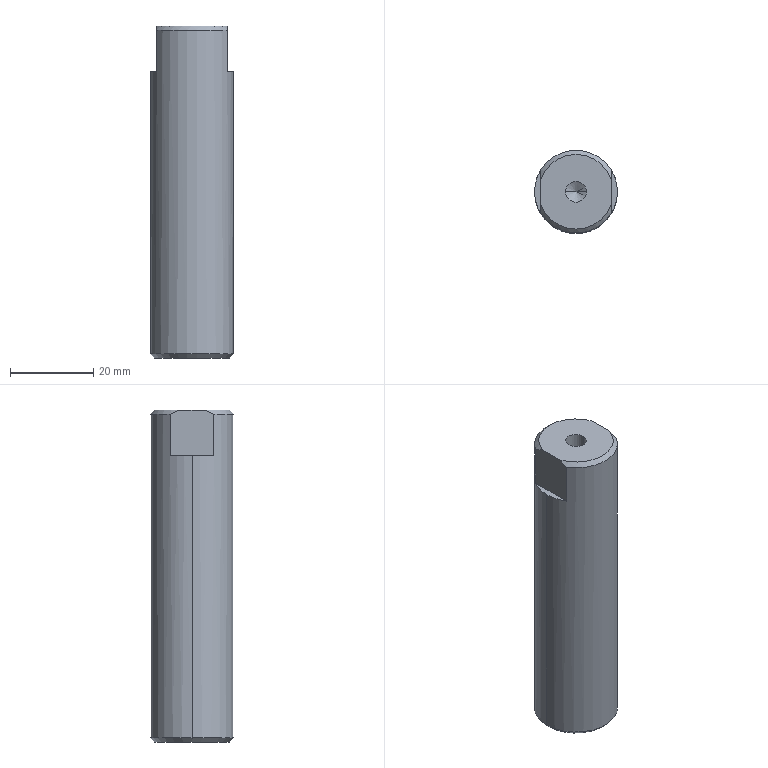Part | STEP file | MT-COMBO-119-S009 | 1 solid | 20 faces | box 20 x 20 x 80 mm | volume 24237 mm3 | cone 8 | cylinder 6 | plane 6 | commonest cylinder face diameters 5 x4 20 x2
STEP:
#1=CARTESIAN_POINT('',(2.5,0.,-65.));
#2=VERTEX_POINT('',#1);
#3=CARTESIAN_POINT('',(-2.5,0.,-65.));
#4=VERTEX_POINT('',#3);
#5=CARTESIAN_POINT('',(0.,0.,-65.));
#6=DIRECTION('',(0.,0.,-1.));
#7=DIRECTION('',(-1.,0.,0.));
#8=AXIS2_PLACEMENT_3D('',#5,#6,#7);
#9=CIRCLE('',#8,2.5);
#10=EDGE_CURVE('',#2,#4,#9,.T.);
#11=ORIENTED_EDGE('',*,*,#10,.F.);
#12=CARTESIAN_POINT('',(2.5,0.,-80.));
#13=VERTEX_POINT('',#12);
#14=CARTESIAN_POINT('',(2.5,0.,-80.));
#15=DIRECTION('',(0.,0.,-1.));
#16=VECTOR('',#15,1000.);
#17=LINE('',#14,#16);
#18=EDGE_CURVE('',#2,#13,#17,.T.);
#19=ORIENTED_EDGE('',*,*,#18,.T.);
#20=CARTESIAN_POINT('',(-2.5,0.,-80.));
#21=VERTEX_POINT('',#20);
#22=CARTESIAN_POINT('',(0.,0.,-80.));
#23=DIRECTION('',(0.,0.,-1.));
#24=DIRECTION('',(-1.,0.,0.));
#25=AXIS2_PLACEMENT_3D('',#22,#23,#24);
#26=CIRCLE('',#25,2.5);
#27=EDGE_CURVE('',#13,#21,#26,.T.);
#28=ORIENTED_EDGE('',*,*,#27,.T.);
#29=CARTESIAN_POINT('',(-2.5,0.,-80.));
#30=DIRECTION('',(0.,0.,-1.));
#31=VECTOR('',#30,1000.);
#32=LINE('',#29,#31);
#33=EDGE_CURVE('',#4,#21,#32,.T.);
#34=ORIENTED_EDGE('',*,*,#33,.F.);
#35=EDGE_LOOP('',(#11,#19,#28,#34));
#36=FACE_OUTER_BOUND('',#35,.T.);
#37=CARTESIAN_POINT('',(0.,0.,-80.));
#38=DIRECTION('',(0.,0.,-1.));
#39=DIRECTION('',(-1.,0.,0.));
#40=AXIS2_PLACEMENT_3D('',#37,#38,#39);
#41=CYLINDRICAL_SURFACE('',#40,2.5);
#42=ADVANCED_FACE('',(#36),#41,.F.);
#43=CARTESIAN_POINT('',(0.,0.,-63.498));
#44=VERTEX_POINT('',#43);
#45=CARTESIAN_POINT('',(-2.5,0.,-65.));
#46=DIRECTION('',(-0.8572,0.,-0.515));
#47=VECTOR('',#46,1000.);
#48=LINE('',#45,#47);
#49=EDGE_CURVE('',#44,#4,#48,.T.);
#50=ORIENTED_EDGE('',*,*,#49,.F.);
#51=CARTESIAN_POINT('',(2.5,0.,-65.));
#52=DIRECTION('',(0.8572,0.,-0.515));
#53=VECTOR('',#52,1000.);
#54=LINE('',#51,#53);
#55=EDGE_CURVE('',#44,#2,#54,.T.);
#56=ORIENTED_EDGE('',*,*,#55,.T.);
#57=ORIENTED_EDGE('',*,*,#10,.T.);
#58=EDGE_LOOP('',(#50,#56,#57));
#59=FACE_OUTER_BOUND('',#58,.T.);
#60=CARTESIAN_POINT('',(0.,0.,-65.));
#61=DIRECTION('',(0.,0.,-1.));
#62=DIRECTION('',(-1.,0.,0.));
#63=AXIS2_PLACEMENT_3D('',#60,#61,#62);
#64=CONICAL_SURFACE('',#63,2.5,1.03);
#65=ADVANCED_FACE('',(#59),#64,.F.);
#66=CARTESIAN_POINT('',(-2.5,0.,-15.));
#67=VERTEX_POINT('',#66);
#68=CARTESIAN_POINT('',(2.5,0.,-15.));
#69=VERTEX_POINT('',#68);
#70=CARTESIAN_POINT('',(0.,0.,-15.));
#71=DIRECTION('',(0.,0.,1.));
#72=DIRECTION('',(1.,0.,0.));
#73=AXIS2_PLACEMENT_3D('',#70,#71,#72);
#74=CIRCLE('',#73,2.5);
#75=EDGE_CURVE('',#67,#69,#74,.T.);
#76=ORIENTED_EDGE('',*,*,#75,.F.);
#77=CARTESIAN_POINT('',(-2.5,0.,0.));
#78=VERTEX_POINT('',#77);
#79=CARTESIAN_POINT('',(-2.5,0.,0.));
#80=DIRECTION('',(0.,0.,1.));
#81=VECTOR('',#80,1000.);
#82=LINE('',#79,#81);
#83=EDGE_CURVE('',#67,#78,#82,.T.);
#84=ORIENTED_EDGE('',*,*,#83,.T.);
#85=CARTESIAN_POINT('',(2.5,0.,0.));
#86=VERTEX_POINT('',#85);
#87=CARTESIAN_POINT('',(0.,0.,0.));
#88=DIRECTION('',(0.,0.,1.));
#89=DIRECTION('',(1.,0.,0.));
#90=AXIS2_PLACEMENT_3D('',#87,#88,#89);
#91=CIRCLE('',#90,2.5);
#92=EDGE_CURVE('',#78,#86,#91,.T.);
#93=ORIENTED_EDGE('',*,*,#92,.T.);
#94=CARTESIAN_POINT('',(2.5,0.,0.));
#95=DIRECTION('',(0.,0.,1.));
#96=VECTOR('',#95,1000.);
#97=LINE('',#94,#96);
#98=EDGE_CURVE('',#69,#86,#97,.T.);
#99=ORIENTED_EDGE('',*,*,#98,.F.);
#100=EDGE_LOOP('',(#76,#84,#93,#99));
#101=FACE_OUTER_BOUND('',#100,.T.);
#102=CARTESIAN_POINT('',(0.,0.,0.));
#103=DIRECTION('',(0.,0.,1.));
#104=DIRECTION('',(1.,0.,0.));
#105=AXIS2_PLACEMENT_3D('',#102,#103,#104);
#106=CYLINDRICAL_SURFACE('',#105,2.5);
#107=ADVANCED_FACE('',(#101),#106,.F.);
#108=CARTESIAN_POINT('',(0.,0.,-16.502));
#109=VERTEX_POINT('',#108);
#110=CARTESIAN_POINT('',(2.5,0.,-15.));
#111=DIRECTION('',(0.8572,0.,0.515));
#112=VECTOR('',#111,1000.);
#113=LINE('',#110,#112);
#114=EDGE_CURVE('',#109,#69,#113,.T.);
#115=ORIENTED_EDGE('',*,*,#114,.F.);
#116=CARTESIAN_POINT('',(-2.5,0.,-15.));
#117=DIRECTION('',(-0.8572,0.,0.515));
#118=VECTOR('',#117,1000.);
#119=LINE('',#116,#118);
#120=EDGE_CURVE('',#109,#67,#119,.T.);
#121=ORIENTED_EDGE('',*,*,#120,.T.);
#122=ORIENTED_EDGE('',*,*,#75,.T.);
#123=EDGE_LOOP('',(#115,#121,#122));
#124=FACE_OUTER_BOUND('',#123,.T.);
#125=CARTESIAN_POINT('',(0.,0.,-15.));
#126=DIRECTION('',(0.,0.,1.));
#127=DIRECTION('',(1.,0.,0.));
#128=AXIS2_PLACEMENT_3D('',#125,#126,#127);
#129=CONICAL_SURFACE('',#128,2.5,1.03);
#130=ADVANCED_FACE('',(#124),#129,.F.);
#131=CARTESIAN_POINT('',(10.,0.,-79.));
#132=VERTEX_POINT('',#131);
#133=CARTESIAN_POINT('',(-10.,0.,-79.));
#134=VERTEX_POINT('',#133);
#135=CARTESIAN_POINT('',(0.,0.,-79.));
#136=DIRECTION('',(0.,0.,-1.));
#137=DIRECTION('',(-1.,0.,0.));
#138=AXIS2_PLACEMENT_3D('',#135,#136,#137);
#139=CIRCLE('',#138,10.);
#140=EDGE_CURVE('',#132,#134,#139,.T.);
#141=ORIENTED_EDGE('',*,*,#140,.F.);
#142=CARTESIAN_POINT('',(10.,0.,-11.));
#143=VERTEX_POINT('',#142);
#144=CARTESIAN_POINT('',(10.,0.,-80.));
#145=DIRECTION('',(0.,0.,1.));
#146=VECTOR('',#145,1000.);
#147=LINE('',#144,#146);
#148=EDGE_CURVE('',#132,#143,#147,.T.);
#149=ORIENTED_EDGE('',*,*,#148,.T.);
#150=CARTESIAN_POINT('',(8.5,-5.268,-11.));
#151=VERTEX_POINT('',#150);
#152=CARTESIAN_POINT('',(0.,0.,-11.));
#153=DIRECTION('',(0.,0.,1.));
#154=DIRECTION('',(1.,0.,0.));
#155=AXIS2_PLACEMENT_3D('',#152,#153,#154);
#156=CIRCLE('',#155,10.);
#157=EDGE_CURVE('',#151,#143,#156,.T.);
#158=ORIENTED_EDGE('',*,*,#157,.F.);
#159=CARTESIAN_POINT('',(8.5,-5.268,-1.));
#160=VERTEX_POINT('',#159);
#161=CARTESIAN_POINT('',(8.5,-5.268,-11.));
#162=DIRECTION('',(0.,0.,1.));
#163=VECTOR('',#162,1000.);
#164=LINE('',#161,#163);
#165=EDGE_CURVE('',#151,#160,#164,.T.);
#166=ORIENTED_EDGE('',*,*,#165,.T.);
#167=CARTESIAN_POINT('',(-8.5,-5.268,-1.));
#168=VERTEX_POINT('',#167);
#169=CARTESIAN_POINT('',(0.,0.,-1.));
#170=DIRECTION('',(0.,0.,-1.));
#171=DIRECTION('',(-1.,0.,0.));
#172=AXIS2_PLACEMENT_3D('',#169,#170,#171);
#173=CIRCLE('',#172,10.);
#174=EDGE_CURVE('',#160,#168,#173,.T.);
#175=ORIENTED_EDGE('',*,*,#174,.T.);
#176=CARTESIAN_POINT('',(-8.5,-5.268,-11.));
#177=VERTEX_POINT('',#176);
#178=CARTESIAN_POINT('',(-8.5,-5.268,-11.));
#179=DIRECTION('',(0.,0.,1.));
#180=VECTOR('',#179,1000.);
#181=LINE('',#178,#180);
#182=EDGE_CURVE('',#177,#168,#181,.T.);
#183=ORIENTED_EDGE('',*,*,#182,.F.);
#184=CARTESIAN_POINT('',(-10.,0.,-11.));
#185=VERTEX_POINT('',#184);
#186=CARTESIAN_POINT('',(0.,0.,-11.));
#187=DIRECTION('',(0.,0.,1.));
#188=DIRECTION('',(1.,0.,0.));
#189=AXIS2_PLACEMENT_3D('',#186,#187,#188);
#190=CIRCLE('',#189,10.);
#191=EDGE_CURVE('',#185,#177,#190,.T.);
#192=ORIENTED_EDGE('',*,*,#191,.F.);
#193=CARTESIAN_POINT('',(-10.,0.,-80.));
#194=DIRECTION('',(0.,0.,1.));
#195=VECTOR('',#194,1000.);
#196=LINE('',#193,#195);
#197=EDGE_CURVE('',#134,#185,#196,.T.);
#198=ORIENTED_EDGE('',*,*,#197,.F.);
#199=EDGE_LOOP('',(#141,#149,#158,#166,#175,#183,#192,#198));
#200=FACE_OUTER_BOUND('',#199,.T.);
#201=CARTESIAN_POINT('',(0.,0.,-80.));
#202=DIRECTION('',(0.,0.,1.));
#203=DIRECTION('',(-1.,0.,0.));
#204=AXIS2_PLACEMENT_3D('',#201,#202,#203);
#205=CYLINDRICAL_SURFACE('',#204,10.);
#206=ADVANCED_FACE('',(#200),#205,.T.);
#207=CARTESIAN_POINT('',(-9.,0.,-80.));
#208=VERTEX_POINT('',#207);
#209=CARTESIAN_POINT('',(9.,0.,-80.));
#210=VERTEX_POINT('',#209);
#211=CARTESIAN_POINT('',(0.,0.,-80.));
#212=DIRECTION('',(0.,0.,-1.));
#213=DIRECTION('',(-1.,0.,0.));
#214=AXIS2_PLACEMENT_3D('',#211,#212,#213);
#215=CIRCLE('',#214,9.);
#216=EDGE_CURVE('',#208,#210,#215,.T.);
#217=ORIENTED_EDGE('',*,*,#216,.F.);
#218=CARTESIAN_POINT('',(-10.,0.,-79.));
#219=DIRECTION('',(-0.7071,0.,0.7071));
#220=VECTOR('',#219,1000.);
#221=LINE('',#218,#220);
#222=EDGE_CURVE('',#208,#134,#221,.T.);
#223=ORIENTED_EDGE('',*,*,#222,.T.);
#224=CARTESIAN_POINT('',(0.,0.,-79.));
#225=DIRECTION('',(0.,0.,-1.));
#226=DIRECTION('',(-1.,0.,0.));
#227=AXIS2_PLACEMENT_3D('',#224,#225,#226);
#228=CIRCLE('',#227,10.);
#229=EDGE_CURVE('',#134,#132,#228,.T.);
#230=ORIENTED_EDGE('',*,*,#229,.T.);
#231=CARTESIAN_POINT('',(10.,0.,-79.));
#232=DIRECTION('',(0.7071,0.,0.7071));
#233=VECTOR('',#232,1000.);
#234=LINE('',#231,#233);
#235=EDGE_CURVE('',#210,#132,#234,.T.);
#236=ORIENTED_EDGE('',*,*,#235,.F.);
#237=EDGE_LOOP('',(#217,#223,#230,#236));
#238=FACE_OUTER_BOUND('',#237,.T.);
#239=CARTESIAN_POINT('',(0.,0.,-79.));
#240=DIRECTION('',(0.,0.,1.));
#241=DIRECTION('',(1.,0.,0.));
#242=AXIS2_PLACEMENT_3D('',#239,#240,#241);
#243=CONICAL_SURFACE('',#242,10.,0.7854);
#244=ADVANCED_FACE('',(#238),#243,.T.);
#245=CARTESIAN_POINT('',(-8.5,2.958,0.));
#246=VERTEX_POINT('',#245);
#247=CARTESIAN_POINT('',(8.5,2.958,0.));
#248=VERTEX_POINT('',#247);
#249=CARTESIAN_POINT('',(0.,0.,0.));
#250=DIRECTION('',(0.,0.,-1.));
#251=DIRECTION('',(-1.,0.,0.));
#252=AXIS2_PLACEMENT_3D('',#249,#250,#251);
#253=CIRCLE('',#252,9.);
#254=EDGE_CURVE('',#246,#248,#253,.T.);
#255=ORIENTED_EDGE('',*,*,#254,.F.);
#256=CARTESIAN_POINT('',(-8.5,-2.958,0.));
#257=VERTEX_POINT('',#256);
#258=CARTESIAN_POINT('',(-8.5,5.268,0.));
#259=DIRECTION('',(0.,-1.,0.));
#260=VECTOR('',#259,1000.);
#261=LINE('',#258,#260);
#262=EDGE_CURVE('',#246,#257,#261,.T.);
#263=ORIENTED_EDGE('',*,*,#262,.T.);
#264=CARTESIAN_POINT('',(8.5,-2.958,0.));
#265=VERTEX_POINT('',#264);
#266=CARTESIAN_POINT('',(0.,0.,0.));
#267=DIRECTION('',(0.,0.,-1.));
#268=DIRECTION('',(-1.,0.,0.));
#269=AXIS2_PLACEMENT_3D('',#266,#267,#268);
#270=CIRCLE('',#269,9.);
#271=EDGE_CURVE('',#265,#257,#270,.T.);
#272=ORIENTED_EDGE('',*,*,#271,.F.);
#273=CARTESIAN_POINT('',(8.5,-5.268,0.));
#274=DIRECTION('',(0.,1.,0.));
#275=VECTOR('',#274,1000.);
#276=LINE('',#273,#275);
#277=EDGE_CURVE('',#265,#248,#276,.T.);
#278=ORIENTED_EDGE('',*,*,#277,.T.);
#279=EDGE_LOOP('',(#255,#263,#272,#278));
#280=FACE_OUTER_BOUND('',#279,.T.);
#281=CARTESIAN_POINT('',(0.,0.,0.));
#282=DIRECTION('',(0.,0.,1.));
#283=DIRECTION('',(1.,0.,0.));
#284=AXIS2_PLACEMENT_3D('',#281,#282,#283);
#285=CIRCLE('',#284,2.5);
#286=EDGE_CURVE('',#86,#78,#285,.T.);
#287=ORIENTED_EDGE('',*,*,#286,.F.);
#288=ORIENTED_EDGE('',*,*,#92,.F.);
#289=EDGE_LOOP('',(#287,#288));
#290=FACE_BOUND('',#289,.T.);
#291=CARTESIAN_POINT('',(0.,0.,0.));
#292=DIRECTION('',(0.,0.,-1.));
#293=DIRECTION('',(0.,-1.,0.));
#294=AXIS2_PLACEMENT_3D('',#291,#292,#293);
#295=PLANE('',#294);
#296=ADVANCED_FACE('',(#280,#290),#295,.F.);
#297=CARTESIAN_POINT('',(8.5,-2.958,0.));
#298=CARTESIAN_POINT('',(8.5,-3.687,-0.2397));
#299=CARTESIAN_POINT('',(8.5,-4.457,-0.5731));
#300=CARTESIAN_POINT('',(8.5,-5.268,-1.));
#301=B_SPLINE_CURVE_WITH_KNOTS('',3,(#297,#298,#299,#300),.UNSPECIFIED.,.F.,.F.,(4,4),(0.,1.),.UNSPECIFIED.);
#302=EDGE_CURVE('',#265,#160,#301,.T.);
#303=ORIENTED_EDGE('',*,*,#302,.F.);
#304=ORIENTED_EDGE('',*,*,#271,.T.);
#305=CARTESIAN_POINT('',(-8.5,-5.268,-1.));
#306=CARTESIAN_POINT('',(-8.5,-4.457,-0.5731));
#307=CARTESIAN_POINT('',(-8.5,-3.687,-0.2397));
#308=CARTESIAN_POINT('',(-8.5,-2.958,0.));
#309=B_SPLINE_CURVE_WITH_KNOTS('',3,(#305,#306,#307,#308),.UNSPECIFIED.,.F.,.F.,(4,4),(0.,1.),.UNSPECIFIED.);
#310=EDGE_CURVE('',#168,#257,#309,.T.);
#311=ORIENTED_EDGE('',*,*,#310,.F.);
#312=ORIENTED_EDGE('',*,*,#174,.F.);
#313=EDGE_LOOP('',(#303,#304,#311,#312));
#314=FACE_OUTER_BOUND('',#313,.T.);
#315=CARTESIAN_POINT('',(0.,0.,0.));
#316=DIRECTION('',(0.,0.,-1.));
#317=DIRECTION('',(-1.,0.,0.));
#318=AXIS2_PLACEMENT_3D('',#315,#316,#317);
#319=CONICAL_SURFACE('',#318,9.,0.7854);
#320=ADVANCED_FACE('',(#314),#319,.T.);
#321=ORIENTED_EDGE('',*,*,#310,.T.);
#322=ORIENTED_EDGE('',*,*,#262,.F.);
#323=CARTESIAN_POINT('',(-8.5,5.268,-1.));
#324=VERTEX_POINT('',#323);
#325=CARTESIAN_POINT('',(-8.5,2.958,0.));
#326=CARTESIAN_POINT('',(-8.5,3.687,-0.2397));
#327=CARTESIAN_POINT('',(-8.5,4.457,-0.5731));
#328=CARTESIAN_POINT('',(-8.5,5.268,-1.));
#329=B_SPLINE_CURVE_WITH_KNOTS('',3,(#325,#326,#327,#328),.UNSPECIFIED.,.F.,.F.,(4,4),(0.,1.),.UNSPECIFIED.);
#330=EDGE_CURVE('',#246,#324,#329,.T.);
#331=ORIENTED_EDGE('',*,*,#330,.T.);
#332=CARTESIAN_POINT('',(-8.5,5.268,-11.));
#333=VERTEX_POINT('',#332);
#334=CARTESIAN_POINT('',(-8.5,5.268,-11.));
#335=DIRECTION('',(0.,0.,1.));
#336=VECTOR('',#335,1000.);
#337=LINE('',#334,#336);
#338=EDGE_CURVE('',#333,#324,#337,.T.);
#339=ORIENTED_EDGE('',*,*,#338,.F.);
#340=CARTESIAN_POINT('',(-8.5,5.268,-11.));
#341=DIRECTION('',(0.,-1.,0.));
#342=VECTOR('',#341,1000.);
#343=LINE('',#340,#342);
#344=EDGE_CURVE('',#333,#177,#343,.T.);
#345=ORIENTED_EDGE('',*,*,#344,.T.);
#346=ORIENTED_EDGE('',*,*,#182,.T.);
#347=EDGE_LOOP('',(#321,#322,#331,#339,#345,#346));
#348=FACE_OUTER_BOUND('',#347,.T.);
#349=CARTESIAN_POINT('',(-8.5,5.268,-11.));
#350=DIRECTION('',(-1.,0.,0.));
#351=DIRECTION('',(0.,0.,1.));
#352=AXIS2_PLACEMENT_3D('',#349,#350,#351);
#353=PLANE('',#352);
#354=ADVANCED_FACE('',(#348),#353,.T.);
#355=CARTESIAN_POINT('',(0.,0.,-80.));
#356=DIRECTION('',(0.,0.,-1.));
#357=DIRECTION('',(-1.,0.,0.));
#358=AXIS2_PLACEMENT_3D('',#355,#356,#357);
#359=CIRCLE('',#358,9.);
#360=EDGE_CURVE('',#210,#208,#359,.T.);
#361=ORIENTED_EDGE('',*,*,#360,.T.);
#362=ORIENTED_EDGE('',*,*,#216,.T.);
#363=EDGE_LOOP('',(#361,#362));
#364=FACE_OUTER_BOUND('',#363,.T.);
#365=CARTESIAN_POINT('',(0.,0.,-80.));
#366=DIRECTION('',(0.,0.,-1.));
#367=DIRECTION('',(-1.,0.,0.));
#368=AXIS2_PLACEMENT_3D('',#365,#366,#367);
#369=CIRCLE('',#368,2.5);
#370=EDGE_CURVE('',#21,#13,#369,.T.);
#371=ORIENTED_EDGE('',*,*,#370,.F.);
#372=ORIENTED_EDGE('',*,*,#27,.F.);
#373=EDGE_LOOP('',(#371,#372));
#374=FACE_BOUND('',#373,.T.);
#375=CARTESIAN_POINT('',(0.,9.,-80.));
#376=DIRECTION('',(0.,0.,1.));
#377=DIRECTION('',(1.,0.,0.));
#378=AXIS2_PLACEMENT_3D('',#375,#376,#377);
#379=PLANE('',#378);
#380=ADVANCED_FACE('',(#364,#374),#379,.F.);
#381=ORIENTED_EDGE('',*,*,#222,.F.);
#382=ORIENTED_EDGE('',*,*,#360,.F.);
#383=ORIENTED_EDGE('',*,*,#235,.T.);
#384=ORIENTED_EDGE('',*,*,#140,.T.);
#385=EDGE_LOOP('',(#381,#382,#383,#384));
#386=FACE_OUTER_BOUND('',#385,.T.);
#387=CARTESIAN_POINT('',(0.,0.,-79.));
#388=DIRECTION('',(0.,0.,1.));
#389=DIRECTION('',(1.,0.,0.));
#390=AXIS2_PLACEMENT_3D('',#387,#388,#389);
#391=CONICAL_SURFACE('',#390,10.,0.7854);
#392=ADVANCED_FACE('',(#386),#391,.T.);
#393=ORIENTED_EDGE('',*,*,#148,.F.);
#394=ORIENTED_EDGE('',*,*,#229,.F.);
#395=ORIENTED_EDGE('',*,*,#197,.T.);
#396=CARTESIAN_POINT('',(0.,0.,-11.));
#397=DIRECTION('',(0.,0.,1.));
#398=DIRECTION('',(1.,0.,0.));
#399=AXIS2_PLACEMENT_3D('',#396,#397,#398);
#400=CIRCLE('',#399,10.);
#401=EDGE_CURVE('',#333,#185,#400,.T.);
#402=ORIENTED_EDGE('',*,*,#401,.F.);
#403=ORIENTED_EDGE('',*,*,#338,.T.);
#404=CARTESIAN_POINT('',(8.5,5.268,-1.));
#405=VERTEX_POINT('',#404);
#406=CARTESIAN_POINT('',(0.,0.,-1.));
#407=DIRECTION('',(0.,0.,-1.));
#408=DIRECTION('',(-1.,0.,0.));
#409=AXIS2_PLACEMENT_3D('',#406,#407,#408);
#410=CIRCLE('',#409,10.);
#411=EDGE_CURVE('',#324,#405,#410,.T.);
#412=ORIENTED_EDGE('',*,*,#411,.T.);
#413=CARTESIAN_POINT('',(8.5,5.268,-11.));
#414=VERTEX_POINT('',#413);
#415=CARTESIAN_POINT('',(8.5,5.268,-11.));
#416=DIRECTION('',(0.,0.,1.));
#417=VECTOR('',#416,1000.);
#418=LINE('',#415,#417);
#419=EDGE_CURVE('',#414,#405,#418,.T.);
#420=ORIENTED_EDGE('',*,*,#419,.F.);
#421=CARTESIAN_POINT('',(0.,0.,-11.));
#422=DIRECTION('',(0.,0.,1.));
#423=DIRECTION('',(1.,0.,0.));
#424=AXIS2_PLACEMENT_3D('',#421,#422,#423);
#425=CIRCLE('',#424,10.);
#426=EDGE_CURVE('',#143,#414,#425,.T.);
#427=ORIENTED_EDGE('',*,*,#426,.F.);
#428=EDGE_LOOP('',(#393,#394,#395,#402,#403,#412,#420,#427));
#429=FACE_OUTER_BOUND('',#428,.T.);
#430=CARTESIAN_POINT('',(0.,0.,-80.));
#431=DIRECTION('',(0.,0.,1.));
#432=DIRECTION('',(-1.,0.,0.));
#433=AXIS2_PLACEMENT_3D('',#430,#431,#432);
#434=CYLINDRICAL_SURFACE('',#433,10.);
#435=ADVANCED_FACE('',(#429),#434,.T.);
#436=ORIENTED_EDGE('',*,*,#330,.F.);
#437=ORIENTED_EDGE('',*,*,#254,.T.);
#438=CARTESIAN_POINT('',(8.5,5.268,-1.));
#439=CARTESIAN_POINT('',(8.5,4.457,-0.5731));
#440=CARTESIAN_POINT('',(8.5,3.687,-0.2397));
#441=CARTESIAN_POINT('',(8.5,2.958,0.));
#442=B_SPLINE_CURVE_WITH_KNOTS('',3,(#438,#439,#440,#441),.UNSPECIFIED.,.F.,.F.,(4,4),(0.,1.),.UNSPECIFIED.);
#443=EDGE_CURVE('',#405,#248,#442,.T.);
#444=ORIENTED_EDGE('',*,*,#443,.F.);
#445=ORIENTED_EDGE('',*,*,#411,.F.);
#446=EDGE_LOOP('',(#436,#437,#444,#445));
#447=FACE_OUTER_BOUND('',#446,.T.);
#448=CARTESIAN_POINT('',(0.,0.,0.));
#449=DIRECTION('',(0.,0.,-1.));
#450=DIRECTION('',(-1.,0.,0.));
#451=AXIS2_PLACEMENT_3D('',#448,#449,#450);
#452=CONICAL_SURFACE('',#451,9.,0.7854);
#453=ADVANCED_FACE('',(#447),#452,.T.);
#454=ORIENTED_EDGE('',*,*,#443,.T.);
#455=ORIENTED_EDGE('',*,*,#277,.F.);
#456=ORIENTED_EDGE('',*,*,#302,.T.);
#457=ORIENTED_EDGE('',*,*,#165,.F.);
#458=CARTESIAN_POINT('',(8.5,-5.268,-11.));
#459=DIRECTION('',(0.,1.,0.));
#460=VECTOR('',#459,1000.);
#461=LINE('',#458,#460);
#462=EDGE_CURVE('',#151,#414,#461,.T.);
#463=ORIENTED_EDGE('',*,*,#462,.T.);
#464=ORIENTED_EDGE('',*,*,#419,.T.);
#465=EDGE_LOOP('',(#454,#455,#456,#457,#463,#464));
#466=FACE_OUTER_BOUND('',#465,.T.);
#467=CARTESIAN_POINT('',(8.5,-5.268,-11.));
#468=DIRECTION('',(1.,0.,0.));
#469=DIRECTION('',(0.,1.,0.));
#470=AXIS2_PLACEMENT_3D('',#467,#468,#469);
#471=PLANE('',#470);
#472=ADVANCED_FACE('',(#466),#471,.T.);
#473=ORIENTED_EDGE('',*,*,#157,.T.);
#474=ORIENTED_EDGE('',*,*,#426,.T.);
#475=ORIENTED_EDGE('',*,*,#462,.F.);
#476=EDGE_LOOP('',(#473,#474,#475));
#477=FACE_OUTER_BOUND('',#476,.T.);
#478=CARTESIAN_POINT('',(0.,0.,-11.));
#479=DIRECTION('',(0.,0.,1.));
#480=DIRECTION('',(1.,0.,0.));
#481=AXIS2_PLACEMENT_3D('',#478,#479,#480);
#482=PLANE('',#481);
#483=ADVANCED_FACE('',(#477),#482,.T.);
#484=ORIENTED_EDGE('',*,*,#401,.T.);
#485=ORIENTED_EDGE('',*,*,#191,.T.);
#486=ORIENTED_EDGE('',*,*,#344,.F.);
#487=EDGE_LOOP('',(#484,#485,#486));
#488=FACE_OUTER_BOUND('',#487,.T.);
#489=CARTESIAN_POINT('',(0.,0.,-11.));
#490=DIRECTION('',(0.,0.,1.));
#491=DIRECTION('',(1.,0.,0.));
#492=AXIS2_PLACEMENT_3D('',#489,#490,#491);
#493=PLANE('',#492);
#494=ADVANCED_FACE('',(#488),#493,.T.);
#495=ORIENTED_EDGE('',*,*,#120,.F.);
#496=ORIENTED_EDGE('',*,*,#114,.T.);
#497=CARTESIAN_POINT('',(0.,0.,-15.));
#498=DIRECTION('',(0.,0.,1.));
#499=DIRECTION('',(1.,0.,0.));
#500=AXIS2_PLACEMENT_3D('',#497,#498,#499);
#501=CIRCLE('',#500,2.5);
#502=EDGE_CURVE('',#69,#67,#501,.T.);
#503=ORIENTED_EDGE('',*,*,#502,.T.);
#504=EDGE_LOOP('',(#495,#496,#503));
#505=FACE_OUTER_BOUND('',#504,.T.);
#506=CARTESIAN_POINT('',(0.,0.,-15.));
#507=DIRECTION('',(0.,0.,1.));
#508=DIRECTION('',(1.,0.,0.));
#509=AXIS2_PLACEMENT_3D('',#506,#507,#508);
#510=CONICAL_SURFACE('',#509,2.5,1.03);
#511=ADVANCED_FACE('',(#505),#510,.F.);
#512=ORIENTED_EDGE('',*,*,#83,.F.);
#513=ORIENTED_EDGE('',*,*,#502,.F.);
#514=ORIENTED_EDGE('',*,*,#98,.T.);
#515=ORIENTED_EDGE('',*,*,#286,.T.);
#516=EDGE_LOOP('',(#512,#513,#514,#515));
#517=FACE_OUTER_BOUND('',#516,.T.);
#518=CARTESIAN_POINT('',(0.,0.,0.));
#519=DIRECTION('',(0.,0.,1.));
#520=DIRECTION('',(1.,0.,0.));
#521=AXIS2_PLACEMENT_3D('',#518,#519,#520);
#522=CYLINDRICAL_SURFACE('',#521,2.5);
#523=ADVANCED_FACE('',(#517),#522,.F.);
#524=ORIENTED_EDGE('',*,*,#55,.F.);
#525=ORIENTED_EDGE('',*,*,#49,.T.);
#526=CARTESIAN_POINT('',(0.,0.,-65.));
#527=DIRECTION('',(0.,0.,-1.));
#528=DIRECTION('',(-1.,0.,0.));
#529=AXIS2_PLACEMENT_3D('',#526,#527,#528);
#530=CIRCLE('',#529,2.5);
#531=EDGE_CURVE('',#4,#2,#530,.T.);
#532=ORIENTED_EDGE('',*,*,#531,.T.);
#533=EDGE_LOOP('',(#524,#525,#532));
#534=FACE_OUTER_BOUND('',#533,.T.);
#535=CARTESIAN_POINT('',(0.,0.,-65.));
#536=DIRECTION('',(0.,0.,-1.));
#537=DIRECTION('',(-1.,0.,0.));
#538=AXIS2_PLACEMENT_3D('',#535,#536,#537);
#539=CONICAL_SURFACE('',#538,2.5,1.03);
#540=ADVANCED_FACE('',(#534),#539,.F.);
#541=ORIENTED_EDGE('',*,*,#18,.F.);
#542=ORIENTED_EDGE('',*,*,#531,.F.);
#543=ORIENTED_EDGE('',*,*,#33,.T.);
#544=ORIENTED_EDGE('',*,*,#370,.T.);
#545=EDGE_LOOP('',(#541,#542,#543,#544));
#546=FACE_OUTER_BOUND('',#545,.T.);
#547=CARTESIAN_POINT('',(0.,0.,-80.));
#548=DIRECTION('',(0.,0.,-1.));
#549=DIRECTION('',(-1.,0.,0.));
#550=AXIS2_PLACEMENT_3D('',#547,#548,#549);
#551=CYLINDRICAL_SURFACE('',#550,2.5);
#552=ADVANCED_FACE('',(#546),#551,.F.);
#553=CLOSED_SHELL('',(#42,#65,#107,#130,#206,#244,#296,#320,#354,#380,#392,#435,#453,#472,#483,#494,#511,#523,#540,#552));
#554=MANIFOLD_SOLID_BREP('',#553);
#555=CARTESIAN_POINT('',(0.,0.,0.));
#556=DIRECTION('',(0.,0.,1.));
#557=DIRECTION('',(1.,0.,0.));
#558=AXIS2_PLACEMENT_3D('',#555,#556,#557);
#559=(LENGTH_UNIT()NAMED_UNIT(*)SI_UNIT(.MILLI.,.METRE.));
#560=UNCERTAINTY_MEASURE_WITH_UNIT(LENGTH_MEASURE(0.00001),#559,'','');
#561=(NAMED_UNIT(*)PLANE_ANGLE_UNIT()SI_UNIT($,.RADIAN.));
#562=(NAMED_UNIT(*)SI_UNIT($,.STERADIAN.)SOLID_ANGLE_UNIT());
#563=(GEOMETRIC_REPRESENTATION_CONTEXT(3)GLOBAL_UNCERTAINTY_ASSIGNED_CONTEXT((#560))GLOBAL_UNIT_ASSIGNED_CONTEXT((#559,#561,#562))REPRESENTATION_CONTEXT('',''));
#564=ADVANCED_BREP_SHAPE_REPRESENTATION('',(#554,#558),#563);